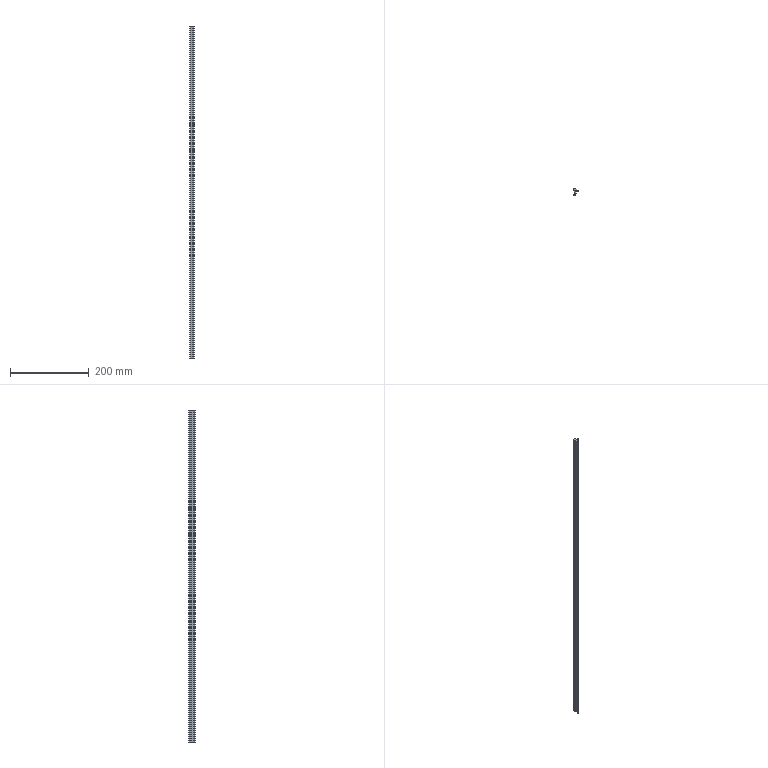Part | SolidWorks | features BaseBody 1, MoveFace 1 | 1 solid | 20 faces | box 10.8 x 17.5 x 842 mm | volume 66350 mm3 | cylinder 11 | plane 9 | commonest cylinder face diameters 1.6 x2 14 x2 0.4 x1 0.6 x1 0.8 x1 2.6 x1
STEP:
#1=CARTESIAN_POINT('',(-3.236,-11.055,742.));
#2=VERTEX_POINT('',#1);
#3=CARTESIAN_POINT('',(-4.3,-10.3,742.));
#4=VERTEX_POINT('',#3);
#5=CARTESIAN_POINT('',(-3.5,-10.3,742.));
#6=DIRECTION('',(0.,0.,-1.));
#7=DIRECTION('',(1.,0.,0.));
#8=AXIS2_PLACEMENT_3D('',#5,#6,#7);
#9=CIRCLE('',#8,0.8);
#10=EDGE_CURVE('',#2,#4,#9,.T.);
#11=ORIENTED_EDGE('',*,*,#10,.T.);
#12=CARTESIAN_POINT('',(-4.3,-10.3,-100.));
#13=VERTEX_POINT('',#12);
#14=CARTESIAN_POINT('',(-4.3,-10.3,-100.));
#15=DIRECTION('',(0.,0.,-1.));
#16=VECTOR('',#15,1000.);
#17=LINE('',#14,#16);
#18=EDGE_CURVE('',#4,#13,#17,.T.);
#19=ORIENTED_EDGE('',*,*,#18,.T.);
#20=CARTESIAN_POINT('',(-3.236,-11.055,-100.));
#21=VERTEX_POINT('',#20);
#22=CARTESIAN_POINT('',(-3.5,-10.3,-100.));
#23=DIRECTION('',(0.,0.,1.));
#24=DIRECTION('',(-1.,0.,0.));
#25=AXIS2_PLACEMENT_3D('',#22,#23,#24);
#26=CIRCLE('',#25,0.8);
#27=EDGE_CURVE('',#13,#21,#26,.T.);
#28=ORIENTED_EDGE('',*,*,#27,.T.);
#29=CARTESIAN_POINT('',(-3.236,-11.055,-100.));
#30=DIRECTION('',(0.,0.,-1.));
#31=VECTOR('',#30,1000.);
#32=LINE('',#29,#31);
#33=EDGE_CURVE('',#2,#21,#32,.T.);
#34=ORIENTED_EDGE('',*,*,#33,.F.);
#35=EDGE_LOOP('',(#11,#19,#28,#34));
#36=FACE_OUTER_BOUND('',#35,.T.);
#37=CARTESIAN_POINT('',(-3.5,-10.3,-100.));
#38=DIRECTION('',(0.,0.,-1.));
#39=DIRECTION('',(-1.,0.,0.));
#40=AXIS2_PLACEMENT_3D('',#37,#38,#39);
#41=CYLINDRICAL_SURFACE('',#40,0.8);
#42=ADVANCED_FACE('',(#36),#41,.T.);
#43=CARTESIAN_POINT('',(1.184,-6.397,-100.));
#44=VERTEX_POINT('',#43);
#45=CARTESIAN_POINT('',(-5.702,-4.29,-100.));
#46=DIRECTION('',(0.,0.,1.));
#47=DIRECTION('',(-1.,0.,0.));
#48=AXIS2_PLACEMENT_3D('',#45,#46,#47);
#49=CIRCLE('',#48,7.201);
#50=EDGE_CURVE('',#21,#44,#49,.T.);
#51=ORIENTED_EDGE('',*,*,#50,.T.);
#52=CARTESIAN_POINT('',(1.184,-6.397,742.));
#53=VERTEX_POINT('',#52);
#54=CARTESIAN_POINT('',(1.184,-6.397,-100.));
#55=DIRECTION('',(0.,0.,1.));
#56=VECTOR('',#55,1000.);
#57=LINE('',#54,#56);
#58=EDGE_CURVE('',#44,#53,#57,.T.);
#59=ORIENTED_EDGE('',*,*,#58,.T.);
#60=CARTESIAN_POINT('',(-5.702,-4.29,742.));
#61=DIRECTION('',(0.,0.,-1.));
#62=DIRECTION('',(1.,0.,0.));
#63=AXIS2_PLACEMENT_3D('',#60,#61,#62);
#64=CIRCLE('',#63,7.201);
#65=EDGE_CURVE('',#53,#2,#64,.T.);
#66=ORIENTED_EDGE('',*,*,#65,.T.);
#67=ORIENTED_EDGE('',*,*,#33,.T.);
#68=EDGE_LOOP('',(#51,#59,#66,#67));
#69=FACE_OUTER_BOUND('',#68,.T.);
#70=CARTESIAN_POINT('',(-5.702,-4.29,-100.));
#71=DIRECTION('',(0.,0.,-1.));
#72=DIRECTION('',(-1.,0.,0.));
#73=AXIS2_PLACEMENT_3D('',#70,#71,#72);
#74=CYLINDRICAL_SURFACE('',#73,7.201);
#75=ADVANCED_FACE('',(#69),#74,.T.);
#76=CARTESIAN_POINT('',(0.9,-6.,-100.));
#77=VERTEX_POINT('',#76);
#78=CARTESIAN_POINT('',(0.9,-6.3,-100.));
#79=DIRECTION('',(0.,0.,1.));
#80=DIRECTION('',(-1.,0.,0.));
#81=AXIS2_PLACEMENT_3D('',#78,#79,#80);
#82=CIRCLE('',#81,0.3);
#83=EDGE_CURVE('',#44,#77,#82,.T.);
#84=ORIENTED_EDGE('',*,*,#83,.T.);
#85=CARTESIAN_POINT('',(0.9,-6.,742.));
#86=VERTEX_POINT('',#85);
#87=CARTESIAN_POINT('',(0.9,-6.,-100.));
#88=DIRECTION('',(0.,0.,1.));
#89=VECTOR('',#88,1000.);
#90=LINE('',#87,#89);
#91=EDGE_CURVE('',#77,#86,#90,.T.);
#92=ORIENTED_EDGE('',*,*,#91,.T.);
#93=CARTESIAN_POINT('',(0.9,-6.3,742.));
#94=DIRECTION('',(0.,0.,-1.));
#95=DIRECTION('',(1.,0.,0.));
#96=AXIS2_PLACEMENT_3D('',#93,#94,#95);
#97=CIRCLE('',#96,0.3);
#98=EDGE_CURVE('',#86,#53,#97,.T.);
#99=ORIENTED_EDGE('',*,*,#98,.T.);
#100=ORIENTED_EDGE('',*,*,#58,.F.);
#101=EDGE_LOOP('',(#84,#92,#99,#100));
#102=FACE_OUTER_BOUND('',#101,.T.);
#103=CARTESIAN_POINT('',(0.9,-6.3,-100.));
#104=DIRECTION('',(0.,0.,-1.));
#105=DIRECTION('',(-1.,0.,0.));
#106=AXIS2_PLACEMENT_3D('',#103,#104,#105);
#107=CYLINDRICAL_SURFACE('',#106,0.3);
#108=ADVANCED_FACE('',(#102),#107,.T.);
#109=CARTESIAN_POINT('',(-2.5,-0.5,-100.));
#110=VERTEX_POINT('',#109);
#111=CARTESIAN_POINT('',(-2.5,-6.153,-100.));
#112=VERTEX_POINT('',#111);
#113=CARTESIAN_POINT('',(-2.5,-6.397,-100.));
#114=DIRECTION('',(0.,-1.,0.));
#115=VECTOR('',#114,1000.);
#116=LINE('',#113,#115);
#117=EDGE_CURVE('',#110,#112,#116,.T.);
#118=ORIENTED_EDGE('',*,*,#117,.F.);
#119=CARTESIAN_POINT('',(-4.2,1.695,-100.));
#120=VERTEX_POINT('',#119);
#121=CARTESIAN_POINT('',(-1.701,1.875,-100.));
#122=DIRECTION('',(0.,0.,1.));
#123=DIRECTION('',(-1.,0.,0.));
#124=AXIS2_PLACEMENT_3D('',#121,#122,#123);
#125=CIRCLE('',#124,2.506);
#126=EDGE_CURVE('',#120,#110,#125,.T.);
#127=ORIENTED_EDGE('',*,*,#126,.F.);
#128=CARTESIAN_POINT('',(-4.2,5.1,-100.));
#129=VERTEX_POINT('',#128);
#130=CARTESIAN_POINT('',(-4.2,-6.397,-100.));
#131=DIRECTION('',(0.,-1.,0.));
#132=VECTOR('',#131,1000.);
#133=LINE('',#130,#132);
#134=EDGE_CURVE('',#129,#120,#133,.T.);
#135=ORIENTED_EDGE('',*,*,#134,.F.);
#136=CARTESIAN_POINT('',(-2.892,6.4,-100.));
#137=VERTEX_POINT('',#136);
#138=CARTESIAN_POINT('',(-2.9,5.1,-100.));
#139=DIRECTION('',(0.,0.,1.));
#140=DIRECTION('',(-1.,0.,0.));
#141=AXIS2_PLACEMENT_3D('',#138,#139,#140);
#142=CIRCLE('',#141,1.3);
#143=EDGE_CURVE('',#137,#129,#142,.T.);
#144=ORIENTED_EDGE('',*,*,#143,.F.);
#145=CARTESIAN_POINT('',(0.5,5.5,-100.));
#146=VERTEX_POINT('',#145);
#147=CARTESIAN_POINT('',(-2.934,-0.5999,-100.));
#148=DIRECTION('',(0.,0.,1.));
#149=DIRECTION('',(-1.,0.,0.));
#150=AXIS2_PLACEMENT_3D('',#147,#148,#149);
#151=CIRCLE('',#150,7.);
#152=EDGE_CURVE('',#146,#137,#151,.T.);
#153=ORIENTED_EDGE('',*,*,#152,.F.);
#154=CARTESIAN_POINT('',(5.5,1.7,-100.));
#155=VERTEX_POINT('',#154);
#156=CARTESIAN_POINT('',(5.5,1.7,-100.));
#157=DIRECTION('',(-0.7962,0.6051,0.));
#158=VECTOR('',#157,1000.);
#159=LINE('',#156,#158);
#160=EDGE_CURVE('',#155,#146,#159,.T.);
#161=ORIENTED_EDGE('',*,*,#160,.F.);
#162=CARTESIAN_POINT('',(6.458,-0.2215,-100.));
#163=VERTEX_POINT('',#162);
#164=CARTESIAN_POINT('',(6.458,-0.2215,-100.));
#165=DIRECTION('',(-0.4462,0.8949,0.));
#166=VECTOR('',#165,1000.);
#167=LINE('',#164,#166);
#168=EDGE_CURVE('',#163,#155,#167,.T.);
#169=ORIENTED_EDGE('',*,*,#168,.F.);
#170=CARTESIAN_POINT('',(5.895,-0.7433,-100.));
#171=VERTEX_POINT('',#170);
#172=CARTESIAN_POINT('',(6.1,-0.4,-100.));
#173=DIRECTION('',(0.,0.,1.));
#174=DIRECTION('',(-1.,0.,0.));
#175=AXIS2_PLACEMENT_3D('',#172,#173,#174);
#176=CIRCLE('',#175,0.4);
#177=EDGE_CURVE('',#171,#163,#176,.T.);
#178=ORIENTED_EDGE('',*,*,#177,.F.);
#179=CARTESIAN_POINT('',(3.,0.,-100.));
#180=VERTEX_POINT('',#179);
#181=CARTESIAN_POINT('',(2.746,-6.995,-100.));
#182=DIRECTION('',(0.,0.,-1.));
#183=DIRECTION('',(-1.,0.,0.));
#184=AXIS2_PLACEMENT_3D('',#181,#182,#183);
#185=CIRCLE('',#184,7.);
#186=EDGE_CURVE('',#180,#171,#185,.T.);
#187=ORIENTED_EDGE('',*,*,#186,.F.);
#188=CARTESIAN_POINT('',(0.,0.,-100.));
#189=VERTEX_POINT('',#188);
#190=CARTESIAN_POINT('',(-6.814,0.,-100.));
#191=DIRECTION('',(1.,0.,0.));
#192=VECTOR('',#191,1000.);
#193=LINE('',#190,#192);
#194=EDGE_CURVE('',#189,#180,#193,.T.);
#195=ORIENTED_EDGE('',*,*,#194,.F.);
#196=CARTESIAN_POINT('',(0.,-5.8,-100.));
#197=VERTEX_POINT('',#196);
#198=CARTESIAN_POINT('',(0.,-6.397,-100.));
#199=DIRECTION('',(0.,1.,0.));
#200=VECTOR('',#199,1000.);
#201=LINE('',#198,#200);
#202=EDGE_CURVE('',#197,#189,#201,.T.);
#203=ORIENTED_EDGE('',*,*,#202,.F.);
#204=CARTESIAN_POINT('',(0.2,-6.,-100.));
#205=VERTEX_POINT('',#204);
#206=CARTESIAN_POINT('',(0.2,-5.8,-100.));
#207=DIRECTION('',(0.,0.,1.));
#208=DIRECTION('',(-1.,0.,0.));
#209=AXIS2_PLACEMENT_3D('',#206,#207,#208);
#210=CIRCLE('',#209,0.2);
#211=EDGE_CURVE('',#197,#205,#210,.T.);
#212=ORIENTED_EDGE('',*,*,#211,.T.);
#213=CARTESIAN_POINT('',(-6.814,-6.,-100.));
#214=DIRECTION('',(-1.,0.,0.));
#215=VECTOR('',#214,1000.);
#216=LINE('',#213,#215);
#217=EDGE_CURVE('',#77,#205,#216,.T.);
#218=ORIENTED_EDGE('',*,*,#217,.F.);
#219=ORIENTED_EDGE('',*,*,#83,.F.);
#220=ORIENTED_EDGE('',*,*,#50,.F.);
#221=ORIENTED_EDGE('',*,*,#27,.F.);
#222=CARTESIAN_POINT('',(-3.998,-9.674,-100.));
#223=VERTEX_POINT('',#222);
#224=CARTESIAN_POINT('',(-3.5,-10.3,-100.));
#225=DIRECTION('',(0.,0.,1.));
#226=DIRECTION('',(-1.,0.,0.));
#227=AXIS2_PLACEMENT_3D('',#224,#225,#226);
#228=CIRCLE('',#227,0.8);
#229=EDGE_CURVE('',#223,#13,#228,.T.);
#230=ORIENTED_EDGE('',*,*,#229,.F.);
#231=CARTESIAN_POINT('',(-6.814,-6.397,-100.));
#232=DIRECTION('',(0.,0.,-1.));
#233=DIRECTION('',(-1.,0.,0.));
#234=AXIS2_PLACEMENT_3D('',#231,#232,#233);
#235=CIRCLE('',#234,4.321);
#236=EDGE_CURVE('',#112,#223,#235,.T.);
#237=ORIENTED_EDGE('',*,*,#236,.F.);
#238=EDGE_LOOP('',(#118,#127,#135,#144,#153,#161,#169,#178,#187,#195,#203,#212,#218,#219,#220,#221,#230,#237));
#239=FACE_OUTER_BOUND('',#238,.T.);
#240=CARTESIAN_POINT('',(-6.814,-6.397,-100.));
#241=DIRECTION('',(0.,0.,1.));
#242=DIRECTION('',(1.,0.,0.));
#243=AXIS2_PLACEMENT_3D('',#240,#241,#242);
#244=PLANE('',#243);
#245=ADVANCED_FACE('',(#239),#244,.F.);
#246=ORIENTED_EDGE('',*,*,#18,.F.);
#247=CARTESIAN_POINT('',(-3.998,-9.674,742.));
#248=VERTEX_POINT('',#247);
#249=CARTESIAN_POINT('',(-3.5,-10.3,742.));
#250=DIRECTION('',(0.,0.,-1.));
#251=DIRECTION('',(1.,0.,0.));
#252=AXIS2_PLACEMENT_3D('',#249,#250,#251);
#253=CIRCLE('',#252,0.8);
#254=EDGE_CURVE('',#4,#248,#253,.T.);
#255=ORIENTED_EDGE('',*,*,#254,.T.);
#256=CARTESIAN_POINT('',(-3.998,-9.674,-100.));
#257=DIRECTION('',(0.,0.,-1.));
#258=VECTOR('',#257,1000.);
#259=LINE('',#256,#258);
#260=EDGE_CURVE('',#248,#223,#259,.T.);
#261=ORIENTED_EDGE('',*,*,#260,.T.);
#262=ORIENTED_EDGE('',*,*,#229,.T.);
#263=EDGE_LOOP('',(#246,#255,#261,#262));
#264=FACE_OUTER_BOUND('',#263,.T.);
#265=CARTESIAN_POINT('',(-3.5,-10.3,-100.));
#266=DIRECTION('',(0.,0.,-1.));
#267=DIRECTION('',(-1.,0.,0.));
#268=AXIS2_PLACEMENT_3D('',#265,#266,#267);
#269=CYLINDRICAL_SURFACE('',#268,0.8);
#270=ADVANCED_FACE('',(#264),#269,.T.);
#271=CARTESIAN_POINT('',(-4.2,1.695,742.));
#272=VERTEX_POINT('',#271);
#273=CARTESIAN_POINT('',(-2.5,-0.5,742.));
#274=VERTEX_POINT('',#273);
#275=CARTESIAN_POINT('',(-1.701,1.875,742.));
#276=DIRECTION('',(0.,0.,1.));
#277=DIRECTION('',(1.,0.,0.));
#278=AXIS2_PLACEMENT_3D('',#275,#276,#277);
#279=CIRCLE('',#278,2.506);
#280=EDGE_CURVE('',#272,#274,#279,.T.);
#281=ORIENTED_EDGE('',*,*,#280,.T.);
#282=CARTESIAN_POINT('',(-2.5,-6.153,742.));
#283=VERTEX_POINT('',#282);
#284=CARTESIAN_POINT('',(-2.5,-6.397,742.));
#285=DIRECTION('',(0.,-1.,0.));
#286=VECTOR('',#285,1000.);
#287=LINE('',#284,#286);
#288=EDGE_CURVE('',#274,#283,#287,.T.);
#289=ORIENTED_EDGE('',*,*,#288,.T.);
#290=CARTESIAN_POINT('',(-6.814,-6.397,742.));
#291=DIRECTION('',(0.,0.,-1.));
#292=DIRECTION('',(1.,0.,0.));
#293=AXIS2_PLACEMENT_3D('',#290,#291,#292);
#294=CIRCLE('',#293,4.321);
#295=EDGE_CURVE('',#283,#248,#294,.T.);
#296=ORIENTED_EDGE('',*,*,#295,.T.);
#297=ORIENTED_EDGE('',*,*,#254,.F.);
#298=ORIENTED_EDGE('',*,*,#10,.F.);
#299=ORIENTED_EDGE('',*,*,#65,.F.);
#300=ORIENTED_EDGE('',*,*,#98,.F.);
#301=CARTESIAN_POINT('',(0.2,-6.,742.));
#302=VERTEX_POINT('',#301);
#303=CARTESIAN_POINT('',(-6.814,-6.,742.));
#304=DIRECTION('',(-1.,0.,0.));
#305=VECTOR('',#304,1000.);
#306=LINE('',#303,#305);
#307=EDGE_CURVE('',#86,#302,#306,.T.);
#308=ORIENTED_EDGE('',*,*,#307,.T.);
#309=CARTESIAN_POINT('',(0.,-5.8,742.));
#310=VERTEX_POINT('',#309);
#311=CARTESIAN_POINT('',(0.2,-5.8,742.));
#312=DIRECTION('',(0.,0.,-1.));
#313=DIRECTION('',(1.,0.,0.));
#314=AXIS2_PLACEMENT_3D('',#311,#312,#313);
#315=CIRCLE('',#314,0.2);
#316=EDGE_CURVE('',#302,#310,#315,.T.);
#317=ORIENTED_EDGE('',*,*,#316,.T.);
#318=CARTESIAN_POINT('',(0.,0.,742.));
#319=VERTEX_POINT('',#318);
#320=CARTESIAN_POINT('',(0.,-6.397,742.));
#321=DIRECTION('',(0.,1.,0.));
#322=VECTOR('',#321,1000.);
#323=LINE('',#320,#322);
#324=EDGE_CURVE('',#310,#319,#323,.T.);
#325=ORIENTED_EDGE('',*,*,#324,.T.);
#326=CARTESIAN_POINT('',(3.,0.,742.));
#327=VERTEX_POINT('',#326);
#328=CARTESIAN_POINT('',(-6.814,0.,742.));
#329=DIRECTION('',(1.,0.,0.));
#330=VECTOR('',#329,1000.);
#331=LINE('',#328,#330);
#332=EDGE_CURVE('',#319,#327,#331,.T.);
#333=ORIENTED_EDGE('',*,*,#332,.T.);
#334=CARTESIAN_POINT('',(5.895,-0.7433,742.));
#335=VERTEX_POINT('',#334);
#336=CARTESIAN_POINT('',(2.746,-6.995,742.));
#337=DIRECTION('',(0.,0.,-1.));
#338=DIRECTION('',(1.,0.,0.));
#339=AXIS2_PLACEMENT_3D('',#336,#337,#338);
#340=CIRCLE('',#339,7.);
#341=EDGE_CURVE('',#327,#335,#340,.T.);
#342=ORIENTED_EDGE('',*,*,#341,.T.);
#343=CARTESIAN_POINT('',(6.458,-0.2215,742.));
#344=VERTEX_POINT('',#343);
#345=CARTESIAN_POINT('',(6.1,-0.4,742.));
#346=DIRECTION('',(0.,0.,-1.));
#347=DIRECTION('',(1.,0.,0.));
#348=AXIS2_PLACEMENT_3D('',#345,#346,#347);
#349=CIRCLE('',#348,0.4);
#350=EDGE_CURVE('',#344,#335,#349,.T.);
#351=ORIENTED_EDGE('',*,*,#350,.F.);
#352=CARTESIAN_POINT('',(5.5,1.7,742.));
#353=VERTEX_POINT('',#352);
#354=CARTESIAN_POINT('',(6.282,0.1323,742.));
#355=DIRECTION('',(-0.4462,0.8949,0.));
#356=VECTOR('',#355,1000.);
#357=LINE('',#354,#356);
#358=EDGE_CURVE('',#344,#353,#357,.T.);
#359=ORIENTED_EDGE('',*,*,#358,.T.);
#360=CARTESIAN_POINT('',(0.5,5.5,742.));
#361=VERTEX_POINT('',#360);
#362=CARTESIAN_POINT('',(1.595,4.668,742.));
#363=DIRECTION('',(-0.7962,0.6051,0.));
#364=VECTOR('',#363,1000.);
#365=LINE('',#362,#364);
#366=EDGE_CURVE('',#353,#361,#365,.T.);
#367=ORIENTED_EDGE('',*,*,#366,.T.);
#368=CARTESIAN_POINT('',(-2.892,6.4,742.));
#369=VERTEX_POINT('',#368);
#370=CARTESIAN_POINT('',(-2.934,-0.5999,742.));
#371=DIRECTION('',(0.,0.,1.));
#372=DIRECTION('',(1.,0.,0.));
#373=AXIS2_PLACEMENT_3D('',#370,#371,#372);
#374=CIRCLE('',#373,7.);
#375=EDGE_CURVE('',#361,#369,#374,.T.);
#376=ORIENTED_EDGE('',*,*,#375,.T.);
#377=CARTESIAN_POINT('',(-4.2,5.1,742.));
#378=VERTEX_POINT('',#377);
#379=CARTESIAN_POINT('',(-2.9,5.1,742.));
#380=DIRECTION('',(0.,0.,1.));
#381=DIRECTION('',(1.,0.,0.));
#382=AXIS2_PLACEMENT_3D('',#379,#380,#381);
#383=CIRCLE('',#382,1.3);
#384=EDGE_CURVE('',#369,#378,#383,.T.);
#385=ORIENTED_EDGE('',*,*,#384,.T.);
#386=CARTESIAN_POINT('',(-4.2,-6.397,742.));
#387=DIRECTION('',(0.,-1.,0.));
#388=VECTOR('',#387,1000.);
#389=LINE('',#386,#388);
#390=EDGE_CURVE('',#378,#272,#389,.T.);
#391=ORIENTED_EDGE('',*,*,#390,.T.);
#392=EDGE_LOOP('',(#281,#289,#296,#297,#298,#299,#300,#308,#317,#325,#333,#342,#351,#359,#367,#376,#385,#391));
#393=FACE_OUTER_BOUND('',#392,.T.);
#394=CARTESIAN_POINT('',(-6.814,-6.397,742.));
#395=DIRECTION('',(0.,0.,1.));
#396=DIRECTION('',(1.,0.,0.));
#397=AXIS2_PLACEMENT_3D('',#394,#395,#396);
#398=PLANE('',#397);
#399=ADVANCED_FACE('',(#393),#398,.T.);
#400=ORIENTED_EDGE('',*,*,#217,.T.);
#401=CARTESIAN_POINT('',(0.2,-6.,-100.));
#402=DIRECTION('',(0.,0.,1.));
#403=VECTOR('',#402,1000.);
#404=LINE('',#401,#403);
#405=EDGE_CURVE('',#205,#302,#404,.T.);
#406=ORIENTED_EDGE('',*,*,#405,.T.);
#407=ORIENTED_EDGE('',*,*,#307,.F.);
#408=ORIENTED_EDGE('',*,*,#91,.F.);
#409=EDGE_LOOP('',(#400,#406,#407,#408));
#410=FACE_OUTER_BOUND('',#409,.T.);
#411=CARTESIAN_POINT('',(0.9,-6.,-100.));
#412=DIRECTION('',(0.,1.,0.));
#413=DIRECTION('',(0.,0.,1.));
#414=AXIS2_PLACEMENT_3D('',#411,#412,#413);
#415=PLANE('',#414);
#416=ADVANCED_FACE('',(#410),#415,.T.);
#417=CARTESIAN_POINT('',(-2.5,-6.153,-100.));
#418=DIRECTION('',(0.,0.,1.));
#419=VECTOR('',#418,1000.);
#420=LINE('',#417,#419);
#421=EDGE_CURVE('',#112,#283,#420,.T.);
#422=ORIENTED_EDGE('',*,*,#421,.F.);
#423=ORIENTED_EDGE('',*,*,#236,.T.);
#424=ORIENTED_EDGE('',*,*,#260,.F.);
#425=ORIENTED_EDGE('',*,*,#295,.F.);
#426=EDGE_LOOP('',(#422,#423,#424,#425));
#427=FACE_OUTER_BOUND('',#426,.T.);
#428=CARTESIAN_POINT('',(-6.814,-6.397,-100.));
#429=DIRECTION('',(0.,0.,-1.));
#430=DIRECTION('',(-1.,0.,0.));
#431=AXIS2_PLACEMENT_3D('',#428,#429,#430);
#432=CYLINDRICAL_SURFACE('',#431,4.321);
#433=ADVANCED_FACE('',(#427),#432,.F.);
#434=ORIENTED_EDGE('',*,*,#117,.T.);
#435=ORIENTED_EDGE('',*,*,#421,.T.);
#436=ORIENTED_EDGE('',*,*,#288,.F.);
#437=CARTESIAN_POINT('',(-2.5,-0.5,-100.));
#438=DIRECTION('',(0.,0.,-1.));
#439=VECTOR('',#438,1000.);
#440=LINE('',#437,#439);
#441=EDGE_CURVE('',#274,#110,#440,.T.);
#442=ORIENTED_EDGE('',*,*,#441,.T.);
#443=EDGE_LOOP('',(#434,#435,#436,#442));
#444=FACE_OUTER_BOUND('',#443,.T.);
#445=CARTESIAN_POINT('',(-2.5,-0.5,-100.));
#446=DIRECTION('',(-1.,0.,0.));
#447=DIRECTION('',(0.,0.,1.));
#448=AXIS2_PLACEMENT_3D('',#445,#446,#447);
#449=PLANE('',#448);
#450=ADVANCED_FACE('',(#444),#449,.T.);
#451=ORIENTED_EDGE('',*,*,#126,.T.);
#452=ORIENTED_EDGE('',*,*,#441,.F.);
#453=ORIENTED_EDGE('',*,*,#280,.F.);
#454=CARTESIAN_POINT('',(-4.2,1.695,-100.));
#455=DIRECTION('',(0.,0.,-1.));
#456=VECTOR('',#455,1000.);
#457=LINE('',#454,#456);
#458=EDGE_CURVE('',#272,#120,#457,.T.);
#459=ORIENTED_EDGE('',*,*,#458,.T.);
#460=EDGE_LOOP('',(#451,#452,#453,#459));
#461=FACE_OUTER_BOUND('',#460,.T.);
#462=CARTESIAN_POINT('',(-1.701,1.875,-100.));
#463=DIRECTION('',(0.,0.,-1.));
#464=DIRECTION('',(-1.,0.,0.));
#465=AXIS2_PLACEMENT_3D('',#462,#463,#464);
#466=CYLINDRICAL_SURFACE('',#465,2.506);
#467=ADVANCED_FACE('',(#461),#466,.T.);
#468=ORIENTED_EDGE('',*,*,#134,.T.);
#469=ORIENTED_EDGE('',*,*,#458,.F.);
#470=ORIENTED_EDGE('',*,*,#390,.F.);
#471=CARTESIAN_POINT('',(-4.2,5.1,-100.));
#472=DIRECTION('',(0.,0.,-1.));
#473=VECTOR('',#472,1000.);
#474=LINE('',#471,#473);
#475=EDGE_CURVE('',#378,#129,#474,.T.);
#476=ORIENTED_EDGE('',*,*,#475,.T.);
#477=EDGE_LOOP('',(#468,#469,#470,#476));
#478=FACE_OUTER_BOUND('',#477,.T.);
#479=CARTESIAN_POINT('',(-4.2,5.1,-100.));
#480=DIRECTION('',(-1.,0.,0.));
#481=DIRECTION('',(0.,0.,1.));
#482=AXIS2_PLACEMENT_3D('',#479,#480,#481);
#483=PLANE('',#482);
#484=ADVANCED_FACE('',(#478),#483,.T.);
#485=ORIENTED_EDGE('',*,*,#143,.T.);
#486=ORIENTED_EDGE('',*,*,#475,.F.);
#487=ORIENTED_EDGE('',*,*,#384,.F.);
#488=CARTESIAN_POINT('',(-2.892,6.4,-100.));
#489=DIRECTION('',(0.,0.,-1.));
#490=VECTOR('',#489,1000.);
#491=LINE('',#488,#490);
#492=EDGE_CURVE('',#369,#137,#491,.T.);
#493=ORIENTED_EDGE('',*,*,#492,.T.);
#494=EDGE_LOOP('',(#485,#486,#487,#493));
#495=FACE_OUTER_BOUND('',#494,.T.);
#496=CARTESIAN_POINT('',(-2.9,5.1,-100.));
#497=DIRECTION('',(0.,0.,-1.));
#498=DIRECTION('',(-1.,0.,0.));
#499=AXIS2_PLACEMENT_3D('',#496,#497,#498);
#500=CYLINDRICAL_SURFACE('',#499,1.3);
#501=ADVANCED_FACE('',(#495),#500,.T.);
#502=ORIENTED_EDGE('',*,*,#152,.T.);
#503=ORIENTED_EDGE('',*,*,#492,.F.);
#504=ORIENTED_EDGE('',*,*,#375,.F.);
#505=CARTESIAN_POINT('',(0.5,5.5,-100.));
#506=DIRECTION('',(0.,0.,-1.));
#507=VECTOR('',#506,1000.);
#508=LINE('',#505,#507);
#509=EDGE_CURVE('',#361,#146,#508,.T.);
#510=ORIENTED_EDGE('',*,*,#509,.T.);
#511=EDGE_LOOP('',(#502,#503,#504,#510));
#512=FACE_OUTER_BOUND('',#511,.T.);
#513=CARTESIAN_POINT('',(-2.934,-0.5999,-100.));
#514=DIRECTION('',(0.,0.,-1.));
#515=DIRECTION('',(-1.,0.,0.));
#516=AXIS2_PLACEMENT_3D('',#513,#514,#515);
#517=CYLINDRICAL_SURFACE('',#516,7.);
#518=ADVANCED_FACE('',(#512),#517,.T.);
#519=ORIENTED_EDGE('',*,*,#160,.T.);
#520=ORIENTED_EDGE('',*,*,#509,.F.);
#521=ORIENTED_EDGE('',*,*,#366,.F.);
#522=CARTESIAN_POINT('',(5.5,1.7,-100.));
#523=DIRECTION('',(0.,0.,-1.));
#524=VECTOR('',#523,1000.);
#525=LINE('',#522,#524);
#526=EDGE_CURVE('',#353,#155,#525,.T.);
#527=ORIENTED_EDGE('',*,*,#526,.T.);
#528=EDGE_LOOP('',(#519,#520,#521,#527));
#529=FACE_OUTER_BOUND('',#528,.T.);
#530=CARTESIAN_POINT('',(5.5,1.7,-100.));
#531=DIRECTION('',(0.6051,0.7962,0.));
#532=DIRECTION('',(-0.7962,0.6051,0.));
#533=AXIS2_PLACEMENT_3D('',#530,#531,#532);
#534=PLANE('',#533);
#535=ADVANCED_FACE('',(#529),#534,.T.);
#536=ORIENTED_EDGE('',*,*,#168,.T.);
#537=ORIENTED_EDGE('',*,*,#526,.F.);
#538=ORIENTED_EDGE('',*,*,#358,.F.);
#539=CARTESIAN_POINT('',(6.458,-0.2215,-100.));
#540=DIRECTION('',(0.,0.,-1.));
#541=VECTOR('',#540,1000.);
#542=LINE('',#539,#541);
#543=EDGE_CURVE('',#344,#163,#542,.T.);
#544=ORIENTED_EDGE('',*,*,#543,.T.);
#545=EDGE_LOOP('',(#536,#537,#538,#544));
#546=FACE_OUTER_BOUND('',#545,.T.);
#547=CARTESIAN_POINT('',(6.458,-0.2215,-100.));
#548=DIRECTION('',(0.8949,0.4462,0.));
#549=DIRECTION('',(-0.4462,0.8949,0.));
#550=AXIS2_PLACEMENT_3D('',#547,#548,#549);
#551=PLANE('',#550);
#552=ADVANCED_FACE('',(#546),#551,.T.);
#553=CARTESIAN_POINT('',(3.,0.,-100.));
#554=DIRECTION('',(0.,0.,1.));
#555=VECTOR('',#554,1000.);
#556=LINE('',#553,#555);
#557=EDGE_CURVE('',#180,#327,#556,.T.);
#558=ORIENTED_EDGE('',*,*,#557,.F.);
#559=ORIENTED_EDGE('',*,*,#186,.T.);
#560=CARTESIAN_POINT('',(5.895,-0.7433,-100.));
#561=DIRECTION('',(0.,0.,-1.));
#562=VECTOR('',#561,1000.);
#563=LINE('',#560,#562);
#564=EDGE_CURVE('',#335,#171,#563,.T.);
#565=ORIENTED_EDGE('',*,*,#564,.F.);
#566=ORIENTED_EDGE('',*,*,#341,.F.);
#567=EDGE_LOOP('',(#558,#559,#565,#566));
#568=FACE_OUTER_BOUND('',#567,.T.);
#569=CARTESIAN_POINT('',(2.746,-6.995,-100.));
#570=DIRECTION('',(0.,0.,-1.));
#571=DIRECTION('',(-1.,0.,0.));
#572=AXIS2_PLACEMENT_3D('',#569,#570,#571);
#573=CYLINDRICAL_SURFACE('',#572,7.);
#574=ADVANCED_FACE('',(#568),#573,.F.);
#575=ORIENTED_EDGE('',*,*,#194,.T.);
#576=ORIENTED_EDGE('',*,*,#557,.T.);
#577=ORIENTED_EDGE('',*,*,#332,.F.);
#578=CARTESIAN_POINT('',(0.,0.,-100.));
#579=DIRECTION('',(0.,0.,-1.));
#580=VECTOR('',#579,1000.);
#581=LINE('',#578,#580);
#582=EDGE_CURVE('',#319,#189,#581,.T.);
#583=ORIENTED_EDGE('',*,*,#582,.T.);
#584=EDGE_LOOP('',(#575,#576,#577,#583));
#585=FACE_OUTER_BOUND('',#584,.T.);
#586=CARTESIAN_POINT('',(0.,0.,-100.));
#587=DIRECTION('',(0.,-1.,0.));
#588=DIRECTION('',(0.,0.,-1.));
#589=AXIS2_PLACEMENT_3D('',#586,#587,#588);
#590=PLANE('',#589);
#591=ADVANCED_FACE('',(#585),#590,.T.);
#592=ORIENTED_EDGE('',*,*,#202,.T.);
#593=ORIENTED_EDGE('',*,*,#582,.F.);
#594=ORIENTED_EDGE('',*,*,#324,.F.);
#595=CARTESIAN_POINT('',(0.,-5.8,-100.));
#596=DIRECTION('',(0.,0.,-1.));
#597=VECTOR('',#596,1000.);
#598=LINE('',#595,#597);
#599=EDGE_CURVE('',#310,#197,#598,.T.);
#600=ORIENTED_EDGE('',*,*,#599,.T.);
#601=EDGE_LOOP('',(#592,#593,#594,#600));
#602=FACE_OUTER_BOUND('',#601,.T.);
#603=CARTESIAN_POINT('',(0.,-5.8,-100.));
#604=DIRECTION('',(1.,0.,0.));
#605=DIRECTION('',(0.,0.,-1.));
#606=AXIS2_PLACEMENT_3D('',#603,#604,#605);
#607=PLANE('',#606);
#608=ADVANCED_FACE('',(#602),#607,.T.);
#609=ORIENTED_EDGE('',*,*,#405,.F.);
#610=ORIENTED_EDGE('',*,*,#211,.F.);
#611=ORIENTED_EDGE('',*,*,#599,.F.);
#612=ORIENTED_EDGE('',*,*,#316,.F.);
#613=EDGE_LOOP('',(#609,#610,#611,#612));
#614=FACE_OUTER_BOUND('',#613,.T.);
#615=CARTESIAN_POINT('',(0.2,-5.8,-100.));
#616=DIRECTION('',(0.,0.,-1.));
#617=DIRECTION('',(-1.,0.,0.));
#618=AXIS2_PLACEMENT_3D('',#615,#616,#617);
#619=CYLINDRICAL_SURFACE('',#618,0.2);
#620=ADVANCED_FACE('',(#614),#619,.F.);
#621=ORIENTED_EDGE('',*,*,#177,.T.);
#622=ORIENTED_EDGE('',*,*,#543,.F.);
#623=ORIENTED_EDGE('',*,*,#350,.T.);
#624=ORIENTED_EDGE('',*,*,#564,.T.);
#625=EDGE_LOOP('',(#621,#622,#623,#624));
#626=FACE_OUTER_BOUND('',#625,.T.);
#627=CARTESIAN_POINT('',(6.1,-0.4,-100.));
#628=DIRECTION('',(0.,0.,-1.));
#629=DIRECTION('',(-1.,0.,0.));
#630=AXIS2_PLACEMENT_3D('',#627,#628,#629);
#631=CYLINDRICAL_SURFACE('',#630,0.4);
#632=ADVANCED_FACE('',(#626),#631,.T.);
#633=CLOSED_SHELL('',(#42,#75,#108,#245,#270,#399,#416,#433,#450,#467,#484,#501,#518,#535,#552,#574,#591,#608,#620,#632));
#634=MANIFOLD_SOLID_BREP('',#633);
#635=CARTESIAN_POINT('',(0.,0.,0.));
#636=DIRECTION('',(0.,0.,1.));
#637=DIRECTION('',(1.,0.,0.));
#638=AXIS2_PLACEMENT_3D('',#635,#636,#637);
#639=(LENGTH_UNIT()NAMED_UNIT(*)SI_UNIT(.MILLI.,.METRE.));
#640=UNCERTAINTY_MEASURE_WITH_UNIT(LENGTH_MEASURE(0.00001),#639,'','');
#641=(NAMED_UNIT(*)PLANE_ANGLE_UNIT()SI_UNIT($,.RADIAN.));
#642=(NAMED_UNIT(*)SI_UNIT($,.STERADIAN.)SOLID_ANGLE_UNIT());
#643=(GEOMETRIC_REPRESENTATION_CONTEXT(3)GLOBAL_UNCERTAINTY_ASSIGNED_CONTEXT((#640))GLOBAL_UNIT_ASSIGNED_CONTEXT((#639,#641,#642))REPRESENTATION_CONTEXT('',''));
#644=ADVANCED_BREP_SHAPE_REPRESENTATION('',(#634,#638),#643);